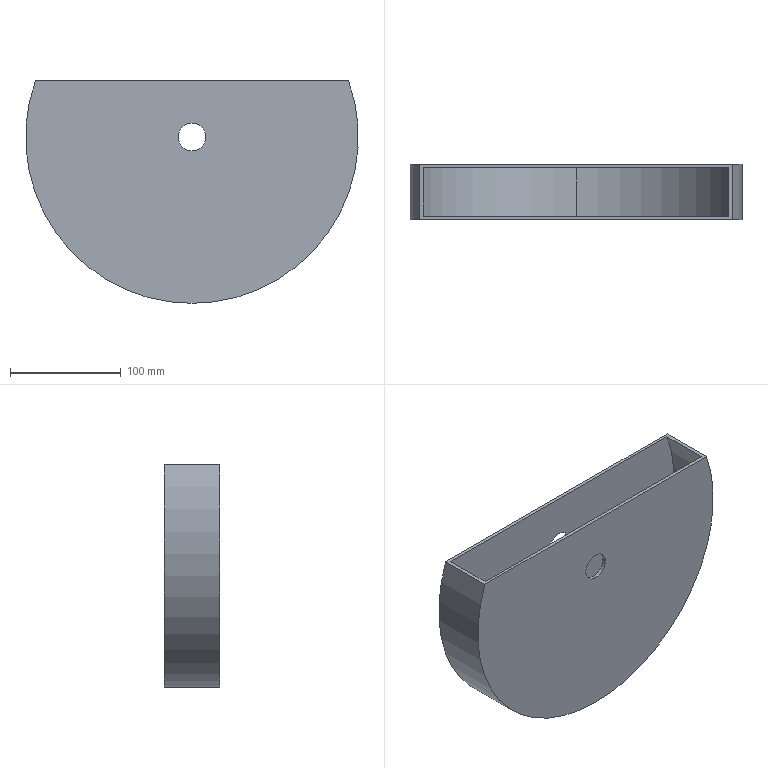Part | SolidWorks | features Extrusion 1, ICE 1, Shell 1 | 1 solid | 13 faces | box 300 x 50 x 200.814 mm | volume 374070 mm3 | cylinder 8 | plane 5 | commonest cylinder face diameters 25 x4 294 x2 300 x2
STEP:
#1=CARTESIAN_POINT('',(0.,47.,-12.5));
#2=VERTEX_POINT('',#1);
#3=CARTESIAN_POINT('',(0.,47.,12.5));
#4=VERTEX_POINT('',#3);
#5=CARTESIAN_POINT('',(0.,47.,0.));
#6=DIRECTION('',(0.,1.,0.));
#7=DIRECTION('',(0.,0.,1.));
#8=AXIS2_PLACEMENT_3D('',#5,#6,#7);
#9=CIRCLE('',#8,12.5);
#10=EDGE_CURVE('',#2,#4,#9,.T.);
#11=ORIENTED_EDGE('',*,*,#10,.F.);
#12=CARTESIAN_POINT('',(0.,50.,-12.5));
#13=VERTEX_POINT('',#12);
#14=CARTESIAN_POINT('',(0.,0.,-12.5));
#15=DIRECTION('',(0.,1.,0.));
#16=VECTOR('',#15,1000.);
#17=LINE('',#14,#16);
#18=EDGE_CURVE('',#2,#13,#17,.T.);
#19=ORIENTED_EDGE('',*,*,#18,.T.);
#20=CARTESIAN_POINT('',(0.,50.,12.5));
#21=VERTEX_POINT('',#20);
#22=CARTESIAN_POINT('',(0.,50.,0.));
#23=DIRECTION('',(0.,1.,0.));
#24=DIRECTION('',(0.,0.,1.));
#25=AXIS2_PLACEMENT_3D('',#22,#23,#24);
#26=CIRCLE('',#25,12.5);
#27=EDGE_CURVE('',#13,#21,#26,.T.);
#28=ORIENTED_EDGE('',*,*,#27,.T.);
#29=CARTESIAN_POINT('',(0.,0.,12.5));
#30=DIRECTION('',(0.,1.,0.));
#31=VECTOR('',#30,1000.);
#32=LINE('',#29,#31);
#33=EDGE_CURVE('',#4,#21,#32,.T.);
#34=ORIENTED_EDGE('',*,*,#33,.F.);
#35=EDGE_LOOP('',(#11,#19,#28,#34));
#36=FACE_OUTER_BOUND('',#35,.T.);
#37=CARTESIAN_POINT('',(0.,0.,0.));
#38=DIRECTION('',(0.,1.,0.));
#39=DIRECTION('',(0.,0.,1.));
#40=AXIS2_PLACEMENT_3D('',#37,#38,#39);
#41=CYLINDRICAL_SURFACE('',#40,12.5);
#42=ADVANCED_FACE('',(#36),#41,.F.);
#43=CARTESIAN_POINT('',(0.,0.,-12.5));
#44=VERTEX_POINT('',#43);
#45=CARTESIAN_POINT('',(0.,0.,12.5));
#46=VERTEX_POINT('',#45);
#47=CARTESIAN_POINT('',(0.,0.,0.));
#48=DIRECTION('',(0.,1.,0.));
#49=DIRECTION('',(0.,0.,1.));
#50=AXIS2_PLACEMENT_3D('',#47,#48,#49);
#51=CIRCLE('',#50,12.5);
#52=EDGE_CURVE('',#44,#46,#51,.T.);
#53=ORIENTED_EDGE('',*,*,#52,.F.);
#54=CARTESIAN_POINT('',(0.,3.,-12.5));
#55=VERTEX_POINT('',#54);
#56=CARTESIAN_POINT('',(0.,0.,-12.5));
#57=DIRECTION('',(0.,1.,0.));
#58=VECTOR('',#57,1000.);
#59=LINE('',#56,#58);
#60=EDGE_CURVE('',#44,#55,#59,.T.);
#61=ORIENTED_EDGE('',*,*,#60,.T.);
#62=CARTESIAN_POINT('',(0.,3.,12.5));
#63=VERTEX_POINT('',#62);
#64=CARTESIAN_POINT('',(0.,3.,0.));
#65=DIRECTION('',(0.,1.,0.));
#66=DIRECTION('',(0.,0.,1.));
#67=AXIS2_PLACEMENT_3D('',#64,#65,#66);
#68=CIRCLE('',#67,12.5);
#69=EDGE_CURVE('',#55,#63,#68,.T.);
#70=ORIENTED_EDGE('',*,*,#69,.T.);
#71=CARTESIAN_POINT('',(0.,0.,12.5));
#72=DIRECTION('',(0.,1.,0.));
#73=VECTOR('',#72,1000.);
#74=LINE('',#71,#73);
#75=EDGE_CURVE('',#46,#63,#74,.T.);
#76=ORIENTED_EDGE('',*,*,#75,.F.);
#77=EDGE_LOOP('',(#53,#61,#70,#76));
#78=FACE_OUTER_BOUND('',#77,.T.);
#79=CARTESIAN_POINT('',(0.,0.,0.));
#80=DIRECTION('',(0.,1.,0.));
#81=DIRECTION('',(0.,0.,1.));
#82=AXIS2_PLACEMENT_3D('',#79,#80,#81);
#83=CYLINDRICAL_SURFACE('',#82,12.5);
#84=ADVANCED_FACE('',(#78),#83,.F.);
#85=CARTESIAN_POINT('',(137.938,47.,50.814));
#86=VERTEX_POINT('',#85);
#87=CARTESIAN_POINT('',(0.,47.,-147.));
#88=VERTEX_POINT('',#87);
#89=CARTESIAN_POINT('',(0.,47.,0.));
#90=DIRECTION('',(0.,1.,0.));
#91=DIRECTION('',(0.,0.,1.));
#92=AXIS2_PLACEMENT_3D('',#89,#90,#91);
#93=CIRCLE('',#92,147.);
#94=EDGE_CURVE('',#86,#88,#93,.T.);
#95=ORIENTED_EDGE('',*,*,#94,.T.);
#96=CARTESIAN_POINT('',(0.,3.,-147.));
#97=VERTEX_POINT('',#96);
#98=CARTESIAN_POINT('',(0.,50.,-147.));
#99=DIRECTION('',(0.,-1.,0.));
#100=VECTOR('',#99,1000.);
#101=LINE('',#98,#100);
#102=EDGE_CURVE('',#88,#97,#101,.T.);
#103=ORIENTED_EDGE('',*,*,#102,.T.);
#104=CARTESIAN_POINT('',(137.938,3.,50.814));
#105=VERTEX_POINT('',#104);
#106=CARTESIAN_POINT('',(0.,3.,0.));
#107=DIRECTION('',(0.,1.,0.));
#108=DIRECTION('',(0.,0.,1.));
#109=AXIS2_PLACEMENT_3D('',#106,#107,#108);
#110=CIRCLE('',#109,147.);
#111=EDGE_CURVE('',#105,#97,#110,.T.);
#112=ORIENTED_EDGE('',*,*,#111,.F.);
#113=CARTESIAN_POINT('',(137.938,47.,50.814));
#114=DIRECTION('',(0.,-1.,0.));
#115=VECTOR('',#114,1000.);
#116=LINE('',#113,#115);
#117=EDGE_CURVE('',#86,#105,#116,.T.);
#118=ORIENTED_EDGE('',*,*,#117,.F.);
#119=EDGE_LOOP('',(#95,#103,#112,#118));
#120=FACE_OUTER_BOUND('',#119,.T.);
#121=CARTESIAN_POINT('',(0.,50.,0.));
#122=DIRECTION('',(0.,-1.,0.));
#123=DIRECTION('',(0.,0.,-1.));
#124=AXIS2_PLACEMENT_3D('',#121,#122,#123);
#125=CYLINDRICAL_SURFACE('',#124,147.);
#126=ADVANCED_FACE('',(#120),#125,.F.);
#127=CARTESIAN_POINT('',(0.,50.,-150.));
#128=VERTEX_POINT('',#127);
#129=CARTESIAN_POINT('',(-141.131,50.,50.814));
#130=VERTEX_POINT('',#129);
#131=CARTESIAN_POINT('',(0.,50.,0.));
#132=DIRECTION('',(0.,1.,0.));
#133=DIRECTION('',(0.,0.,1.));
#134=AXIS2_PLACEMENT_3D('',#131,#132,#133);
#135=CIRCLE('',#134,150.);
#136=EDGE_CURVE('',#128,#130,#135,.T.);
#137=ORIENTED_EDGE('',*,*,#136,.F.);
#138=CARTESIAN_POINT('',(0.,0.,-150.));
#139=VERTEX_POINT('',#138);
#140=CARTESIAN_POINT('',(0.,50.,-150.));
#141=DIRECTION('',(0.,-1.,0.));
#142=VECTOR('',#141,1000.);
#143=LINE('',#140,#142);
#144=EDGE_CURVE('',#128,#139,#143,.T.);
#145=ORIENTED_EDGE('',*,*,#144,.T.);
#146=CARTESIAN_POINT('',(-141.131,0.,50.814));
#147=VERTEX_POINT('',#146);
#148=CARTESIAN_POINT('',(0.,0.,0.));
#149=DIRECTION('',(0.,1.,0.));
#150=DIRECTION('',(0.,0.,1.));
#151=AXIS2_PLACEMENT_3D('',#148,#149,#150);
#152=CIRCLE('',#151,150.);
#153=EDGE_CURVE('',#139,#147,#152,.T.);
#154=ORIENTED_EDGE('',*,*,#153,.T.);
#155=CARTESIAN_POINT('',(-141.131,50.,50.814));
#156=DIRECTION('',(0.,-1.,0.));
#157=VECTOR('',#156,1000.);
#158=LINE('',#155,#157);
#159=EDGE_CURVE('',#130,#147,#158,.T.);
#160=ORIENTED_EDGE('',*,*,#159,.F.);
#161=EDGE_LOOP('',(#137,#145,#154,#160));
#162=FACE_OUTER_BOUND('',#161,.T.);
#163=CARTESIAN_POINT('',(0.,50.,0.));
#164=DIRECTION('',(0.,-1.,0.));
#165=DIRECTION('',(0.,0.,-1.));
#166=AXIS2_PLACEMENT_3D('',#163,#164,#165);
#167=CYLINDRICAL_SURFACE('',#166,150.);
#168=ADVANCED_FACE('',(#162),#167,.T.);
#169=CARTESIAN_POINT('',(141.131,0.,50.814));
#170=VERTEX_POINT('',#169);
#171=CARTESIAN_POINT('',(-141.131,0.,50.814));
#172=DIRECTION('',(1.,0.,0.));
#173=VECTOR('',#172,1000.);
#174=LINE('',#171,#173);
#175=EDGE_CURVE('',#147,#170,#174,.T.);
#176=ORIENTED_EDGE('',*,*,#175,.T.);
#177=CARTESIAN_POINT('',(141.131,50.,50.814));
#178=VERTEX_POINT('',#177);
#179=CARTESIAN_POINT('',(141.131,50.,50.814));
#180=DIRECTION('',(0.,-1.,0.));
#181=VECTOR('',#180,1000.);
#182=LINE('',#179,#181);
#183=EDGE_CURVE('',#178,#170,#182,.T.);
#184=ORIENTED_EDGE('',*,*,#183,.F.);
#185=CARTESIAN_POINT('',(-141.131,50.,50.814));
#186=DIRECTION('',(1.,0.,0.));
#187=VECTOR('',#186,1000.);
#188=LINE('',#185,#187);
#189=EDGE_CURVE('',#130,#178,#188,.T.);
#190=ORIENTED_EDGE('',*,*,#189,.F.);
#191=ORIENTED_EDGE('',*,*,#159,.T.);
#192=EDGE_LOOP('',(#176,#184,#190,#191));
#193=FACE_OUTER_BOUND('',#192,.T.);
#194=CARTESIAN_POINT('',(-137.938,3.,50.814));
#195=VERTEX_POINT('',#194);
#196=CARTESIAN_POINT('',(-141.131,3.,50.814));
#197=DIRECTION('',(1.,0.,0.));
#198=VECTOR('',#197,1000.);
#199=LINE('',#196,#198);
#200=EDGE_CURVE('',#195,#105,#199,.T.);
#201=ORIENTED_EDGE('',*,*,#200,.F.);
#202=CARTESIAN_POINT('',(-137.938,47.,50.814));
#203=VERTEX_POINT('',#202);
#204=CARTESIAN_POINT('',(-137.938,47.,50.814));
#205=DIRECTION('',(0.,-1.,0.));
#206=VECTOR('',#205,1000.);
#207=LINE('',#204,#206);
#208=EDGE_CURVE('',#203,#195,#207,.T.);
#209=ORIENTED_EDGE('',*,*,#208,.F.);
#210=CARTESIAN_POINT('',(-141.131,47.,50.814));
#211=DIRECTION('',(1.,0.,0.));
#212=VECTOR('',#211,1000.);
#213=LINE('',#210,#212);
#214=EDGE_CURVE('',#203,#86,#213,.T.);
#215=ORIENTED_EDGE('',*,*,#214,.T.);
#216=ORIENTED_EDGE('',*,*,#117,.T.);
#217=EDGE_LOOP('',(#201,#209,#215,#216));
#218=FACE_BOUND('',#217,.T.);
#219=CARTESIAN_POINT('',(-141.131,50.,50.814));
#220=DIRECTION('',(0.,0.,-1.));
#221=DIRECTION('',(-1.,0.,0.));
#222=AXIS2_PLACEMENT_3D('',#219,#220,#221);
#223=PLANE('',#222);
#224=ADVANCED_FACE('',(#193,#218),#223,.F.);
#225=ORIENTED_EDGE('',*,*,#144,.F.);
#226=CARTESIAN_POINT('',(0.,50.,0.));
#227=DIRECTION('',(0.,1.,0.));
#228=DIRECTION('',(0.,0.,1.));
#229=AXIS2_PLACEMENT_3D('',#226,#227,#228);
#230=CIRCLE('',#229,150.);
#231=EDGE_CURVE('',#178,#128,#230,.T.);
#232=ORIENTED_EDGE('',*,*,#231,.F.);
#233=ORIENTED_EDGE('',*,*,#183,.T.);
#234=CARTESIAN_POINT('',(0.,0.,0.));
#235=DIRECTION('',(0.,1.,0.));
#236=DIRECTION('',(0.,0.,1.));
#237=AXIS2_PLACEMENT_3D('',#234,#235,#236);
#238=CIRCLE('',#237,150.);
#239=EDGE_CURVE('',#170,#139,#238,.T.);
#240=ORIENTED_EDGE('',*,*,#239,.T.);
#241=EDGE_LOOP('',(#225,#232,#233,#240));
#242=FACE_OUTER_BOUND('',#241,.T.);
#243=CARTESIAN_POINT('',(0.,50.,0.));
#244=DIRECTION('',(0.,-1.,0.));
#245=DIRECTION('',(0.,0.,-1.));
#246=AXIS2_PLACEMENT_3D('',#243,#244,#245);
#247=CYLINDRICAL_SURFACE('',#246,150.);
#248=ADVANCED_FACE('',(#242),#247,.T.);
#249=CARTESIAN_POINT('',(0.,50.,0.));
#250=DIRECTION('',(0.,1.,0.));
#251=DIRECTION('',(0.,0.,1.));
#252=AXIS2_PLACEMENT_3D('',#249,#250,#251);
#253=CIRCLE('',#252,12.5);
#254=EDGE_CURVE('',#21,#13,#253,.T.);
#255=ORIENTED_EDGE('',*,*,#254,.F.);
#256=ORIENTED_EDGE('',*,*,#27,.F.);
#257=EDGE_LOOP('',(#255,#256));
#258=FACE_BOUND('',#257,.T.);
#259=ORIENTED_EDGE('',*,*,#231,.T.);
#260=ORIENTED_EDGE('',*,*,#136,.T.);
#261=ORIENTED_EDGE('',*,*,#189,.T.);
#262=EDGE_LOOP('',(#259,#260,#261));
#263=FACE_OUTER_BOUND('',#262,.T.);
#264=CARTESIAN_POINT('',(0.,50.,0.));
#265=DIRECTION('',(0.,1.,0.));
#266=DIRECTION('',(0.,0.,1.));
#267=AXIS2_PLACEMENT_3D('',#264,#265,#266);
#268=PLANE('',#267);
#269=ADVANCED_FACE('',(#258,#263),#268,.T.);
#270=CARTESIAN_POINT('',(0.,0.,0.));
#271=DIRECTION('',(0.,1.,0.));
#272=DIRECTION('',(0.,0.,1.));
#273=AXIS2_PLACEMENT_3D('',#270,#271,#272);
#274=CIRCLE('',#273,12.5);
#275=EDGE_CURVE('',#46,#44,#274,.T.);
#276=ORIENTED_EDGE('',*,*,#275,.T.);
#277=ORIENTED_EDGE('',*,*,#52,.T.);
#278=EDGE_LOOP('',(#276,#277));
#279=FACE_BOUND('',#278,.T.);
#280=ORIENTED_EDGE('',*,*,#239,.F.);
#281=ORIENTED_EDGE('',*,*,#175,.F.);
#282=ORIENTED_EDGE('',*,*,#153,.F.);
#283=EDGE_LOOP('',(#280,#281,#282));
#284=FACE_OUTER_BOUND('',#283,.T.);
#285=CARTESIAN_POINT('',(0.,0.,0.));
#286=DIRECTION('',(0.,1.,0.));
#287=DIRECTION('',(0.,0.,1.));
#288=AXIS2_PLACEMENT_3D('',#285,#286,#287);
#289=PLANE('',#288);
#290=ADVANCED_FACE('',(#279,#284),#289,.F.);
#291=ORIENTED_EDGE('',*,*,#102,.F.);
#292=CARTESIAN_POINT('',(0.,47.,0.));
#293=DIRECTION('',(0.,1.,0.));
#294=DIRECTION('',(0.,0.,1.));
#295=AXIS2_PLACEMENT_3D('',#292,#293,#294);
#296=CIRCLE('',#295,147.);
#297=EDGE_CURVE('',#88,#203,#296,.T.);
#298=ORIENTED_EDGE('',*,*,#297,.T.);
#299=ORIENTED_EDGE('',*,*,#208,.T.);
#300=CARTESIAN_POINT('',(0.,3.,0.));
#301=DIRECTION('',(0.,1.,0.));
#302=DIRECTION('',(0.,0.,1.));
#303=AXIS2_PLACEMENT_3D('',#300,#301,#302);
#304=CIRCLE('',#303,147.);
#305=EDGE_CURVE('',#97,#195,#304,.T.);
#306=ORIENTED_EDGE('',*,*,#305,.F.);
#307=EDGE_LOOP('',(#291,#298,#299,#306));
#308=FACE_OUTER_BOUND('',#307,.T.);
#309=CARTESIAN_POINT('',(0.,50.,0.));
#310=DIRECTION('',(0.,-1.,0.));
#311=DIRECTION('',(0.,0.,-1.));
#312=AXIS2_PLACEMENT_3D('',#309,#310,#311);
#313=CYLINDRICAL_SURFACE('',#312,147.);
#314=ADVANCED_FACE('',(#308),#313,.F.);
#315=CARTESIAN_POINT('',(0.,47.,0.));
#316=DIRECTION('',(0.,1.,0.));
#317=DIRECTION('',(0.,0.,1.));
#318=AXIS2_PLACEMENT_3D('',#315,#316,#317);
#319=CIRCLE('',#318,12.5);
#320=EDGE_CURVE('',#4,#2,#319,.T.);
#321=ORIENTED_EDGE('',*,*,#320,.T.);
#322=ORIENTED_EDGE('',*,*,#10,.T.);
#323=EDGE_LOOP('',(#321,#322));
#324=FACE_BOUND('',#323,.T.);
#325=ORIENTED_EDGE('',*,*,#94,.F.);
#326=ORIENTED_EDGE('',*,*,#214,.F.);
#327=ORIENTED_EDGE('',*,*,#297,.F.);
#328=EDGE_LOOP('',(#325,#326,#327));
#329=FACE_OUTER_BOUND('',#328,.T.);
#330=CARTESIAN_POINT('',(0.,47.,0.));
#331=DIRECTION('',(0.,1.,0.));
#332=DIRECTION('',(0.,0.,1.));
#333=AXIS2_PLACEMENT_3D('',#330,#331,#332);
#334=PLANE('',#333);
#335=ADVANCED_FACE('',(#324,#329),#334,.F.);
#336=CARTESIAN_POINT('',(0.,3.,0.));
#337=DIRECTION('',(0.,1.,0.));
#338=DIRECTION('',(0.,0.,1.));
#339=AXIS2_PLACEMENT_3D('',#336,#337,#338);
#340=CIRCLE('',#339,12.5);
#341=EDGE_CURVE('',#63,#55,#340,.T.);
#342=ORIENTED_EDGE('',*,*,#341,.F.);
#343=ORIENTED_EDGE('',*,*,#69,.F.);
#344=EDGE_LOOP('',(#342,#343));
#345=FACE_BOUND('',#344,.T.);
#346=ORIENTED_EDGE('',*,*,#111,.T.);
#347=ORIENTED_EDGE('',*,*,#305,.T.);
#348=ORIENTED_EDGE('',*,*,#200,.T.);
#349=EDGE_LOOP('',(#346,#347,#348));
#350=FACE_OUTER_BOUND('',#349,.T.);
#351=CARTESIAN_POINT('',(0.,3.,0.));
#352=DIRECTION('',(0.,1.,0.));
#353=DIRECTION('',(0.,0.,1.));
#354=AXIS2_PLACEMENT_3D('',#351,#352,#353);
#355=PLANE('',#354);
#356=ADVANCED_FACE('',(#345,#350),#355,.T.);
#357=ORIENTED_EDGE('',*,*,#60,.F.);
#358=ORIENTED_EDGE('',*,*,#275,.F.);
#359=ORIENTED_EDGE('',*,*,#75,.T.);
#360=ORIENTED_EDGE('',*,*,#341,.T.);
#361=EDGE_LOOP('',(#357,#358,#359,#360));
#362=FACE_OUTER_BOUND('',#361,.T.);
#363=CARTESIAN_POINT('',(0.,0.,0.));
#364=DIRECTION('',(0.,1.,0.));
#365=DIRECTION('',(0.,0.,1.));
#366=AXIS2_PLACEMENT_3D('',#363,#364,#365);
#367=CYLINDRICAL_SURFACE('',#366,12.5);
#368=ADVANCED_FACE('',(#362),#367,.F.);
#369=ORIENTED_EDGE('',*,*,#18,.F.);
#370=ORIENTED_EDGE('',*,*,#320,.F.);
#371=ORIENTED_EDGE('',*,*,#33,.T.);
#372=ORIENTED_EDGE('',*,*,#254,.T.);
#373=EDGE_LOOP('',(#369,#370,#371,#372));
#374=FACE_OUTER_BOUND('',#373,.T.);
#375=CARTESIAN_POINT('',(0.,0.,0.));
#376=DIRECTION('',(0.,1.,0.));
#377=DIRECTION('',(0.,0.,1.));
#378=AXIS2_PLACEMENT_3D('',#375,#376,#377);
#379=CYLINDRICAL_SURFACE('',#378,12.5);
#380=ADVANCED_FACE('',(#374),#379,.F.);
#381=CLOSED_SHELL('',(#42,#84,#126,#168,#224,#248,#269,#290,#314,#335,#356,#368,#380));
#382=MANIFOLD_SOLID_BREP('',#381);
#383=CARTESIAN_POINT('',(0.,0.,0.));
#384=DIRECTION('',(0.,0.,1.));
#385=DIRECTION('',(1.,0.,0.));
#386=AXIS2_PLACEMENT_3D('',#383,#384,#385);
#387=(LENGTH_UNIT()NAMED_UNIT(*)SI_UNIT(.MILLI.,.METRE.));
#388=UNCERTAINTY_MEASURE_WITH_UNIT(LENGTH_MEASURE(0.00001),#387,'','');
#389=(NAMED_UNIT(*)PLANE_ANGLE_UNIT()SI_UNIT($,.RADIAN.));
#390=(NAMED_UNIT(*)SI_UNIT($,.STERADIAN.)SOLID_ANGLE_UNIT());
#391=(GEOMETRIC_REPRESENTATION_CONTEXT(3)GLOBAL_UNCERTAINTY_ASSIGNED_CONTEXT((#388))GLOBAL_UNIT_ASSIGNED_CONTEXT((#387,#389,#390))REPRESENTATION_CONTEXT('',''));
#392=ADVANCED_BREP_SHAPE_REPRESENTATION('',(#382,#386),#391);